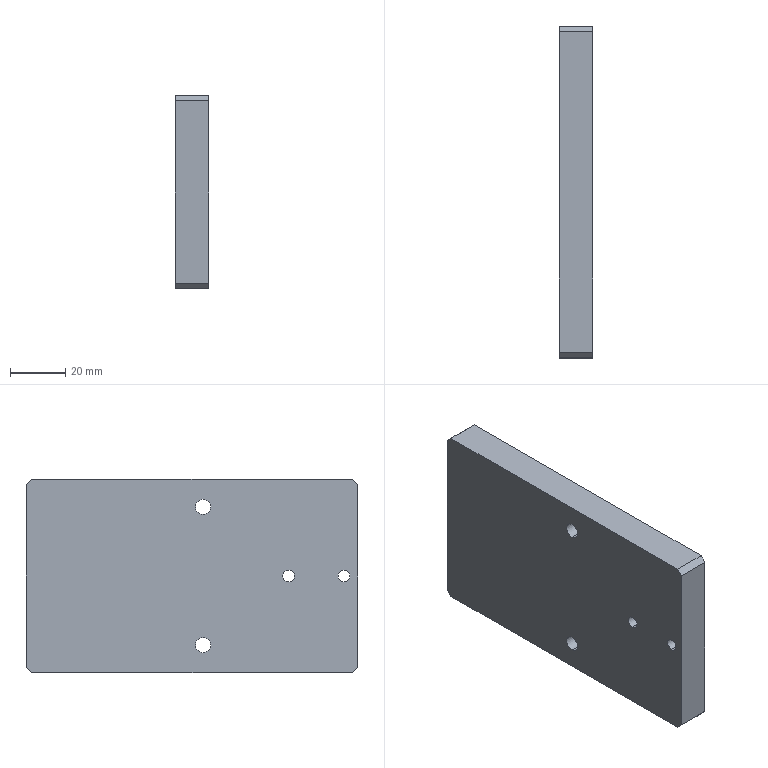Part | SolidWorks | features HoleWzd 4, Chamfer 1, Extrusion 1 | 1 solid | 44 faces | box 12 x 120 x 70 mm | volume 98575 mm3 | cylinder 22 | plane 12 | cone 10 | commonest cylinder face diameters 3.3 x6 4.2 x4 5 x4 5.5 x4 10 x4
STEP:
#1=CARTESIAN_POINT('',(4.,35.5,-26.5));
#2=VERTEX_POINT('',#1);
#3=CARTESIAN_POINT('',(4.,35.5,-31.5));
#4=VERTEX_POINT('',#3);
#5=CARTESIAN_POINT('',(4.,35.5,-29.));
#6=DIRECTION('',(1.,0.,0.));
#7=DIRECTION('',(0.,0.,-1.));
#8=AXIS2_PLACEMENT_3D('',#5,#6,#7);
#9=CIRCLE('',#8,2.5);
#10=EDGE_CURVE('',#2,#4,#9,.T.);
#11=ORIENTED_EDGE('',*,*,#10,.F.);
#12=CARTESIAN_POINT('',(12.,35.5,-26.5));
#13=VERTEX_POINT('',#12);
#14=CARTESIAN_POINT('',(12.,35.5,-26.5));
#15=DIRECTION('',(1.,0.,0.));
#16=VECTOR('',#15,1000.);
#17=LINE('',#14,#16);
#18=EDGE_CURVE('',#2,#13,#17,.T.);
#19=ORIENTED_EDGE('',*,*,#18,.T.);
#20=CARTESIAN_POINT('',(12.,35.5,-31.5));
#21=VERTEX_POINT('',#20);
#22=CARTESIAN_POINT('',(12.,35.5,-29.));
#23=DIRECTION('',(1.,0.,0.));
#24=DIRECTION('',(0.,0.,-1.));
#25=AXIS2_PLACEMENT_3D('',#22,#23,#24);
#26=CIRCLE('',#25,2.5);
#27=EDGE_CURVE('',#13,#21,#26,.T.);
#28=ORIENTED_EDGE('',*,*,#27,.T.);
#29=CARTESIAN_POINT('',(12.,35.5,-31.5));
#30=DIRECTION('',(1.,0.,0.));
#31=VECTOR('',#30,1000.);
#32=LINE('',#29,#31);
#33=EDGE_CURVE('',#4,#21,#32,.T.);
#34=ORIENTED_EDGE('',*,*,#33,.F.);
#35=EDGE_LOOP('',(#11,#19,#28,#34));
#36=FACE_OUTER_BOUND('',#35,.T.);
#37=CARTESIAN_POINT('',(12.,35.5,-29.));
#38=DIRECTION('',(1.,0.,0.));
#39=DIRECTION('',(0.,0.,-1.));
#40=AXIS2_PLACEMENT_3D('',#37,#38,#39);
#41=CYLINDRICAL_SURFACE('',#40,2.5);
#42=ADVANCED_FACE('',(#36),#41,.F.);
#43=CARTESIAN_POINT('',(2.498,35.5,-29.));
#44=VERTEX_POINT('',#43);
#45=CARTESIAN_POINT('',(4.,35.5,-31.5));
#46=DIRECTION('',(0.515,0.,-0.8572));
#47=VECTOR('',#46,1000.);
#48=LINE('',#45,#47);
#49=EDGE_CURVE('',#44,#4,#48,.T.);
#50=ORIENTED_EDGE('',*,*,#49,.F.);
#51=CARTESIAN_POINT('',(4.,35.5,-26.5));
#52=DIRECTION('',(0.515,0.,0.8572));
#53=VECTOR('',#52,1000.);
#54=LINE('',#51,#53);
#55=EDGE_CURVE('',#44,#2,#54,.T.);
#56=ORIENTED_EDGE('',*,*,#55,.T.);
#57=ORIENTED_EDGE('',*,*,#10,.T.);
#58=EDGE_LOOP('',(#50,#56,#57));
#59=FACE_OUTER_BOUND('',#58,.T.);
#60=CARTESIAN_POINT('',(4.,35.5,-29.));
#61=DIRECTION('',(1.,0.,0.));
#62=DIRECTION('',(0.,0.,-1.));
#63=AXIS2_PLACEMENT_3D('',#60,#61,#62);
#64=CONICAL_SURFACE('',#63,2.5,1.03);
#65=ADVANCED_FACE('',(#59),#64,.F.);
#66=CARTESIAN_POINT('',(4.,-12.5,-26.5));
#67=VERTEX_POINT('',#66);
#68=CARTESIAN_POINT('',(4.,-12.5,-31.5));
#69=VERTEX_POINT('',#68);
#70=CARTESIAN_POINT('',(4.,-12.5,-29.));
#71=DIRECTION('',(1.,0.,0.));
#72=DIRECTION('',(0.,0.,-1.));
#73=AXIS2_PLACEMENT_3D('',#70,#71,#72);
#74=CIRCLE('',#73,2.5);
#75=EDGE_CURVE('',#67,#69,#74,.T.);
#76=ORIENTED_EDGE('',*,*,#75,.F.);
#77=CARTESIAN_POINT('',(12.,-12.5,-26.5));
#78=VERTEX_POINT('',#77);
#79=CARTESIAN_POINT('',(12.,-12.5,-26.5));
#80=DIRECTION('',(1.,0.,0.));
#81=VECTOR('',#80,1000.);
#82=LINE('',#79,#81);
#83=EDGE_CURVE('',#67,#78,#82,.T.);
#84=ORIENTED_EDGE('',*,*,#83,.T.);
#85=CARTESIAN_POINT('',(12.,-12.5,-31.5));
#86=VERTEX_POINT('',#85);
#87=CARTESIAN_POINT('',(12.,-12.5,-29.));
#88=DIRECTION('',(1.,0.,0.));
#89=DIRECTION('',(0.,0.,-1.));
#90=AXIS2_PLACEMENT_3D('',#87,#88,#89);
#91=CIRCLE('',#90,2.5);
#92=EDGE_CURVE('',#78,#86,#91,.T.);
#93=ORIENTED_EDGE('',*,*,#92,.T.);
#94=CARTESIAN_POINT('',(12.,-12.5,-31.5));
#95=DIRECTION('',(1.,0.,0.));
#96=VECTOR('',#95,1000.);
#97=LINE('',#94,#96);
#98=EDGE_CURVE('',#69,#86,#97,.T.);
#99=ORIENTED_EDGE('',*,*,#98,.F.);
#100=EDGE_LOOP('',(#76,#84,#93,#99));
#101=FACE_OUTER_BOUND('',#100,.T.);
#102=CARTESIAN_POINT('',(12.,-12.5,-29.));
#103=DIRECTION('',(1.,0.,0.));
#104=DIRECTION('',(0.,0.,-1.));
#105=AXIS2_PLACEMENT_3D('',#102,#103,#104);
#106=CYLINDRICAL_SURFACE('',#105,2.5);
#107=ADVANCED_FACE('',(#101),#106,.F.);
#108=CARTESIAN_POINT('',(2.498,-12.5,-29.));
#109=VERTEX_POINT('',#108);
#110=CARTESIAN_POINT('',(4.,-12.5,-31.5));
#111=DIRECTION('',(0.515,0.,-0.8572));
#112=VECTOR('',#111,1000.);
#113=LINE('',#110,#112);
#114=EDGE_CURVE('',#109,#69,#113,.T.);
#115=ORIENTED_EDGE('',*,*,#114,.F.);
#116=CARTESIAN_POINT('',(4.,-12.5,-26.5));
#117=DIRECTION('',(0.515,0.,0.8572));
#118=VECTOR('',#117,1000.);
#119=LINE('',#116,#118);
#120=EDGE_CURVE('',#109,#67,#119,.T.);
#121=ORIENTED_EDGE('',*,*,#120,.T.);
#122=ORIENTED_EDGE('',*,*,#75,.T.);
#123=EDGE_LOOP('',(#115,#121,#122));
#124=FACE_OUTER_BOUND('',#123,.T.);
#125=CARTESIAN_POINT('',(4.,-12.5,-29.));
#126=DIRECTION('',(1.,0.,0.));
#127=DIRECTION('',(0.,0.,-1.));
#128=AXIS2_PLACEMENT_3D('',#125,#126,#127);
#129=CONICAL_SURFACE('',#128,2.5,1.03);
#130=ADVANCED_FACE('',(#124),#129,.F.);
#131=CARTESIAN_POINT('',(1.9,-48.5,1.65));
#132=VERTEX_POINT('',#131);
#133=CARTESIAN_POINT('',(1.9,-48.5,-1.65));
#134=VERTEX_POINT('',#133);
#135=CARTESIAN_POINT('',(1.9,-48.5,0.));
#136=DIRECTION('',(1.,0.,0.));
#137=DIRECTION('',(0.,0.,-1.));
#138=AXIS2_PLACEMENT_3D('',#135,#136,#137);
#139=CIRCLE('',#138,1.65);
#140=EDGE_CURVE('',#132,#134,#139,.T.);
#141=ORIENTED_EDGE('',*,*,#140,.F.);
#142=CARTESIAN_POINT('',(12.,-48.5,1.65));
#143=VERTEX_POINT('',#142);
#144=CARTESIAN_POINT('',(12.,-48.5,1.65));
#145=DIRECTION('',(1.,0.,0.));
#146=VECTOR('',#145,1000.);
#147=LINE('',#144,#146);
#148=EDGE_CURVE('',#132,#143,#147,.T.);
#149=ORIENTED_EDGE('',*,*,#148,.T.);
#150=CARTESIAN_POINT('',(12.,-48.5,-1.65));
#151=VERTEX_POINT('',#150);
#152=CARTESIAN_POINT('',(12.,-48.5,0.));
#153=DIRECTION('',(1.,0.,0.));
#154=DIRECTION('',(0.,0.,-1.));
#155=AXIS2_PLACEMENT_3D('',#152,#153,#154);
#156=CIRCLE('',#155,1.65);
#157=EDGE_CURVE('',#143,#151,#156,.T.);
#158=ORIENTED_EDGE('',*,*,#157,.T.);
#159=CARTESIAN_POINT('',(12.,-48.5,-1.65));
#160=DIRECTION('',(1.,0.,0.));
#161=VECTOR('',#160,1000.);
#162=LINE('',#159,#161);
#163=EDGE_CURVE('',#134,#151,#162,.T.);
#164=ORIENTED_EDGE('',*,*,#163,.F.);
#165=EDGE_LOOP('',(#141,#149,#158,#164));
#166=FACE_OUTER_BOUND('',#165,.T.);
#167=CARTESIAN_POINT('',(12.,-48.5,0.));
#168=DIRECTION('',(1.,0.,0.));
#169=DIRECTION('',(0.,0.,-1.));
#170=AXIS2_PLACEMENT_3D('',#167,#168,#169);
#171=CYLINDRICAL_SURFACE('',#170,1.65);
#172=ADVANCED_FACE('',(#166),#171,.F.);
#173=CARTESIAN_POINT('',(0.9086,-48.5,0.));
#174=VERTEX_POINT('',#173);
#175=CARTESIAN_POINT('',(1.9,-48.5,-1.65));
#176=DIRECTION('',(0.515,0.,-0.8572));
#177=VECTOR('',#176,1000.);
#178=LINE('',#175,#177);
#179=EDGE_CURVE('',#174,#134,#178,.T.);
#180=ORIENTED_EDGE('',*,*,#179,.F.);
#181=CARTESIAN_POINT('',(1.9,-48.5,1.65));
#182=DIRECTION('',(0.515,0.,0.8572));
#183=VECTOR('',#182,1000.);
#184=LINE('',#181,#183);
#185=EDGE_CURVE('',#174,#132,#184,.T.);
#186=ORIENTED_EDGE('',*,*,#185,.T.);
#187=ORIENTED_EDGE('',*,*,#140,.T.);
#188=EDGE_LOOP('',(#180,#186,#187));
#189=FACE_OUTER_BOUND('',#188,.T.);
#190=CARTESIAN_POINT('',(1.9,-48.5,0.));
#191=DIRECTION('',(1.,0.,0.));
#192=DIRECTION('',(0.,0.,-1.));
#193=AXIS2_PLACEMENT_3D('',#190,#191,#192);
#194=CONICAL_SURFACE('',#193,1.65,1.03);
#195=ADVANCED_FACE('',(#189),#194,.F.);
#196=CARTESIAN_POINT('',(1.9,-12.5,1.65));
#197=VERTEX_POINT('',#196);
#198=CARTESIAN_POINT('',(1.9,-12.5,-1.65));
#199=VERTEX_POINT('',#198);
#200=CARTESIAN_POINT('',(1.9,-12.5,0.));
#201=DIRECTION('',(1.,0.,0.));
#202=DIRECTION('',(0.,0.,-1.));
#203=AXIS2_PLACEMENT_3D('',#200,#201,#202);
#204=CIRCLE('',#203,1.65);
#205=EDGE_CURVE('',#197,#199,#204,.T.);
#206=ORIENTED_EDGE('',*,*,#205,.F.);
#207=CARTESIAN_POINT('',(12.,-12.5,1.65));
#208=VERTEX_POINT('',#207);
#209=CARTESIAN_POINT('',(12.,-12.5,1.65));
#210=DIRECTION('',(1.,0.,0.));
#211=VECTOR('',#210,1000.);
#212=LINE('',#209,#211);
#213=EDGE_CURVE('',#197,#208,#212,.T.);
#214=ORIENTED_EDGE('',*,*,#213,.T.);
#215=CARTESIAN_POINT('',(12.,-12.5,-1.65));
#216=VERTEX_POINT('',#215);
#217=CARTESIAN_POINT('',(12.,-12.5,0.));
#218=DIRECTION('',(1.,0.,0.));
#219=DIRECTION('',(0.,0.,-1.));
#220=AXIS2_PLACEMENT_3D('',#217,#218,#219);
#221=CIRCLE('',#220,1.65);
#222=EDGE_CURVE('',#208,#216,#221,.T.);
#223=ORIENTED_EDGE('',*,*,#222,.T.);
#224=CARTESIAN_POINT('',(12.,-12.5,-1.65));
#225=DIRECTION('',(1.,0.,0.));
#226=VECTOR('',#225,1000.);
#227=LINE('',#224,#226);
#228=EDGE_CURVE('',#199,#216,#227,.T.);
#229=ORIENTED_EDGE('',*,*,#228,.F.);
#230=EDGE_LOOP('',(#206,#214,#223,#229));
#231=FACE_OUTER_BOUND('',#230,.T.);
#232=CARTESIAN_POINT('',(12.,-12.5,0.));
#233=DIRECTION('',(1.,0.,0.));
#234=DIRECTION('',(0.,0.,-1.));
#235=AXIS2_PLACEMENT_3D('',#232,#233,#234);
#236=CYLINDRICAL_SURFACE('',#235,1.65);
#237=ADVANCED_FACE('',(#231),#236,.F.);
#238=CARTESIAN_POINT('',(0.9086,-12.5,0.));
#239=VERTEX_POINT('',#238);
#240=CARTESIAN_POINT('',(1.9,-12.5,-1.65));
#241=DIRECTION('',(0.515,0.,-0.8572));
#242=VECTOR('',#241,1000.);
#243=LINE('',#240,#242);
#244=EDGE_CURVE('',#239,#199,#243,.T.);
#245=ORIENTED_EDGE('',*,*,#244,.F.);
#246=CARTESIAN_POINT('',(1.9,-12.5,1.65));
#247=DIRECTION('',(0.515,0.,0.8572));
#248=VECTOR('',#247,1000.);
#249=LINE('',#246,#248);
#250=EDGE_CURVE('',#239,#197,#249,.T.);
#251=ORIENTED_EDGE('',*,*,#250,.T.);
#252=ORIENTED_EDGE('',*,*,#205,.T.);
#253=EDGE_LOOP('',(#245,#251,#252));
#254=FACE_OUTER_BOUND('',#253,.T.);
#255=CARTESIAN_POINT('',(1.9,-12.5,0.));
#256=DIRECTION('',(1.,0.,0.));
#257=DIRECTION('',(0.,0.,-1.));
#258=AXIS2_PLACEMENT_3D('',#255,#256,#257);
#259=CONICAL_SURFACE('',#258,1.65,1.03);
#260=ADVANCED_FACE('',(#254),#259,.F.);
#261=CARTESIAN_POINT('',(1.9,35.5,1.65));
#262=VERTEX_POINT('',#261);
#263=CARTESIAN_POINT('',(1.9,35.5,-1.65));
#264=VERTEX_POINT('',#263);
#265=CARTESIAN_POINT('',(1.9,35.5,0.));
#266=DIRECTION('',(1.,0.,0.));
#267=DIRECTION('',(0.,0.,-1.));
#268=AXIS2_PLACEMENT_3D('',#265,#266,#267);
#269=CIRCLE('',#268,1.65);
#270=EDGE_CURVE('',#262,#264,#269,.T.);
#271=ORIENTED_EDGE('',*,*,#270,.F.);
#272=CARTESIAN_POINT('',(12.,35.5,1.65));
#273=VERTEX_POINT('',#272);
#274=CARTESIAN_POINT('',(12.,35.5,1.65));
#275=DIRECTION('',(1.,0.,0.));
#276=VECTOR('',#275,1000.);
#277=LINE('',#274,#276);
#278=EDGE_CURVE('',#262,#273,#277,.T.);
#279=ORIENTED_EDGE('',*,*,#278,.T.);
#280=CARTESIAN_POINT('',(12.,35.5,-1.65));
#281=VERTEX_POINT('',#280);
#282=CARTESIAN_POINT('',(12.,35.5,0.));
#283=DIRECTION('',(1.,0.,0.));
#284=DIRECTION('',(0.,0.,-1.));
#285=AXIS2_PLACEMENT_3D('',#282,#283,#284);
#286=CIRCLE('',#285,1.65);
#287=EDGE_CURVE('',#273,#281,#286,.T.);
#288=ORIENTED_EDGE('',*,*,#287,.T.);
#289=CARTESIAN_POINT('',(12.,35.5,-1.65));
#290=DIRECTION('',(1.,0.,0.));
#291=VECTOR('',#290,1000.);
#292=LINE('',#289,#291);
#293=EDGE_CURVE('',#264,#281,#292,.T.);
#294=ORIENTED_EDGE('',*,*,#293,.F.);
#295=EDGE_LOOP('',(#271,#279,#288,#294));
#296=FACE_OUTER_BOUND('',#295,.T.);
#297=CARTESIAN_POINT('',(12.,35.5,0.));
#298=DIRECTION('',(1.,0.,0.));
#299=DIRECTION('',(0.,0.,-1.));
#300=AXIS2_PLACEMENT_3D('',#297,#298,#299);
#301=CYLINDRICAL_SURFACE('',#300,1.65);
#302=ADVANCED_FACE('',(#296),#301,.F.);
#303=CARTESIAN_POINT('',(0.9086,35.5,0.));
#304=VERTEX_POINT('',#303);
#305=CARTESIAN_POINT('',(1.9,35.5,-1.65));
#306=DIRECTION('',(0.515,0.,-0.8572));
#307=VECTOR('',#306,1000.);
#308=LINE('',#305,#307);
#309=EDGE_CURVE('',#304,#264,#308,.T.);
#310=ORIENTED_EDGE('',*,*,#309,.F.);
#311=CARTESIAN_POINT('',(1.9,35.5,1.65));
#312=DIRECTION('',(0.515,0.,0.8572));
#313=VECTOR('',#312,1000.);
#314=LINE('',#311,#313);
#315=EDGE_CURVE('',#304,#262,#314,.T.);
#316=ORIENTED_EDGE('',*,*,#315,.T.);
#317=ORIENTED_EDGE('',*,*,#270,.T.);
#318=EDGE_LOOP('',(#310,#316,#317));
#319=FACE_OUTER_BOUND('',#318,.T.);
#320=CARTESIAN_POINT('',(1.9,35.5,0.));
#321=DIRECTION('',(1.,0.,0.));
#322=DIRECTION('',(0.,0.,-1.));
#323=AXIS2_PLACEMENT_3D('',#320,#321,#322);
#324=CONICAL_SURFACE('',#323,1.65,1.03);
#325=ADVANCED_FACE('',(#319),#324,.F.);
#326=CARTESIAN_POINT('',(6.3,-4.,-20.));
#327=VERTEX_POINT('',#326);
#328=CARTESIAN_POINT('',(6.3,-4.,-30.));
#329=VERTEX_POINT('',#328);
#330=CARTESIAN_POINT('',(6.3,-4.,-25.));
#331=DIRECTION('',(1.,0.,0.));
#332=DIRECTION('',(0.,0.,-1.));
#333=AXIS2_PLACEMENT_3D('',#330,#331,#332);
#334=CIRCLE('',#333,5.);
#335=EDGE_CURVE('',#327,#329,#334,.T.);
#336=ORIENTED_EDGE('',*,*,#335,.F.);
#337=CARTESIAN_POINT('',(12.,-4.,-20.));
#338=VERTEX_POINT('',#337);
#339=CARTESIAN_POINT('',(12.,-4.,-20.));
#340=DIRECTION('',(1.,0.,0.));
#341=VECTOR('',#340,1000.);
#342=LINE('',#339,#341);
#343=EDGE_CURVE('',#327,#338,#342,.T.);
#344=ORIENTED_EDGE('',*,*,#343,.T.);
#345=CARTESIAN_POINT('',(12.,-4.,-30.));
#346=VERTEX_POINT('',#345);
#347=CARTESIAN_POINT('',(12.,-4.,-25.));
#348=DIRECTION('',(1.,0.,0.));
#349=DIRECTION('',(0.,0.,-1.));
#350=AXIS2_PLACEMENT_3D('',#347,#348,#349);
#351=CIRCLE('',#350,5.);
#352=EDGE_CURVE('',#338,#346,#351,.T.);
#353=ORIENTED_EDGE('',*,*,#352,.T.);
#354=CARTESIAN_POINT('',(12.,-4.,-30.));
#355=DIRECTION('',(1.,0.,0.));
#356=VECTOR('',#355,1000.);
#357=LINE('',#354,#356);
#358=EDGE_CURVE('',#329,#346,#357,.T.);
#359=ORIENTED_EDGE('',*,*,#358,.F.);
#360=EDGE_LOOP('',(#336,#344,#353,#359));
#361=FACE_OUTER_BOUND('',#360,.T.);
#362=CARTESIAN_POINT('',(12.,-4.,-25.));
#363=DIRECTION('',(1.,0.,0.));
#364=DIRECTION('',(0.,0.,-1.));
#365=AXIS2_PLACEMENT_3D('',#362,#363,#364);
#366=CYLINDRICAL_SURFACE('',#365,5.);
#367=ADVANCED_FACE('',(#361),#366,.F.);
#368=CARTESIAN_POINT('',(0.,-4.,-22.25));
#369=VERTEX_POINT('',#368);
#370=CARTESIAN_POINT('',(0.,-4.,-27.75));
#371=VERTEX_POINT('',#370);
#372=CARTESIAN_POINT('',(0.,-4.,-25.));
#373=DIRECTION('',(1.,0.,0.));
#374=DIRECTION('',(0.,0.,-1.));
#375=AXIS2_PLACEMENT_3D('',#372,#373,#374);
#376=CIRCLE('',#375,2.75);
#377=EDGE_CURVE('',#369,#371,#376,.T.);
#378=ORIENTED_EDGE('',*,*,#377,.F.);
#379=CARTESIAN_POINT('',(6.3,-4.,-22.25));
#380=VERTEX_POINT('',#379);
#381=CARTESIAN_POINT('',(12.,-4.,-22.25));
#382=DIRECTION('',(1.,0.,0.));
#383=VECTOR('',#382,1000.);
#384=LINE('',#381,#383);
#385=EDGE_CURVE('',#369,#380,#384,.T.);
#386=ORIENTED_EDGE('',*,*,#385,.T.);
#387=CARTESIAN_POINT('',(6.3,-4.,-27.75));
#388=VERTEX_POINT('',#387);
#389=CARTESIAN_POINT('',(6.3,-4.,-25.));
#390=DIRECTION('',(1.,0.,0.));
#391=DIRECTION('',(0.,0.,-1.));
#392=AXIS2_PLACEMENT_3D('',#389,#390,#391);
#393=CIRCLE('',#392,2.75);
#394=EDGE_CURVE('',#380,#388,#393,.T.);
#395=ORIENTED_EDGE('',*,*,#394,.T.);
#396=CARTESIAN_POINT('',(12.,-4.,-27.75));
#397=DIRECTION('',(1.,0.,0.));
#398=VECTOR('',#397,1000.);
#399=LINE('',#396,#398);
#400=EDGE_CURVE('',#371,#388,#399,.T.);
#401=ORIENTED_EDGE('',*,*,#400,.F.);
#402=EDGE_LOOP('',(#378,#386,#395,#401));
#403=FACE_OUTER_BOUND('',#402,.T.);
#404=CARTESIAN_POINT('',(12.,-4.,-25.));
#405=DIRECTION('',(1.,0.,0.));
#406=DIRECTION('',(0.,0.,-1.));
#407=AXIS2_PLACEMENT_3D('',#404,#405,#406);
#408=CYLINDRICAL_SURFACE('',#407,2.75);
#409=ADVANCED_FACE('',(#403),#408,.F.);
#410=CARTESIAN_POINT('',(6.3,-4.,30.));
#411=VERTEX_POINT('',#410);
#412=CARTESIAN_POINT('',(6.3,-4.,20.));
#413=VERTEX_POINT('',#412);
#414=CARTESIAN_POINT('',(6.3,-4.,25.));
#415=DIRECTION('',(1.,0.,0.));
#416=DIRECTION('',(0.,0.,-1.));
#417=AXIS2_PLACEMENT_3D('',#414,#415,#416);
#418=CIRCLE('',#417,5.);
#419=EDGE_CURVE('',#411,#413,#418,.T.);
#420=ORIENTED_EDGE('',*,*,#419,.F.);
#421=CARTESIAN_POINT('',(12.,-4.,30.));
#422=VERTEX_POINT('',#421);
#423=CARTESIAN_POINT('',(12.,-4.,30.));
#424=DIRECTION('',(1.,0.,0.));
#425=VECTOR('',#424,1000.);
#426=LINE('',#423,#425);
#427=EDGE_CURVE('',#411,#422,#426,.T.);
#428=ORIENTED_EDGE('',*,*,#427,.T.);
#429=CARTESIAN_POINT('',(12.,-4.,20.));
#430=VERTEX_POINT('',#429);
#431=CARTESIAN_POINT('',(12.,-4.,25.));
#432=DIRECTION('',(1.,0.,0.));
#433=DIRECTION('',(0.,0.,-1.));
#434=AXIS2_PLACEMENT_3D('',#431,#432,#433);
#435=CIRCLE('',#434,5.);
#436=EDGE_CURVE('',#422,#430,#435,.T.);
#437=ORIENTED_EDGE('',*,*,#436,.T.);
#438=CARTESIAN_POINT('',(12.,-4.,20.));
#439=DIRECTION('',(1.,0.,0.));
#440=VECTOR('',#439,1000.);
#441=LINE('',#438,#440);
#442=EDGE_CURVE('',#413,#430,#441,.T.);
#443=ORIENTED_EDGE('',*,*,#442,.F.);
#444=EDGE_LOOP('',(#420,#428,#437,#443));
#445=FACE_OUTER_BOUND('',#444,.T.);
#446=CARTESIAN_POINT('',(12.,-4.,25.));
#447=DIRECTION('',(1.,0.,0.));
#448=DIRECTION('',(0.,0.,-1.));
#449=AXIS2_PLACEMENT_3D('',#446,#447,#448);
#450=CYLINDRICAL_SURFACE('',#449,5.);
#451=ADVANCED_FACE('',(#445),#450,.F.);
#452=CARTESIAN_POINT('',(0.,-4.,27.75));
#453=VERTEX_POINT('',#452);
#454=CARTESIAN_POINT('',(0.,-4.,22.25));
#455=VERTEX_POINT('',#454);
#456=CARTESIAN_POINT('',(0.,-4.,25.));
#457=DIRECTION('',(1.,0.,0.));
#458=DIRECTION('',(0.,0.,-1.));
#459=AXIS2_PLACEMENT_3D('',#456,#457,#458);
#460=CIRCLE('',#459,2.75);
#461=EDGE_CURVE('',#453,#455,#460,.T.);
#462=ORIENTED_EDGE('',*,*,#461,.F.);
#463=CARTESIAN_POINT('',(6.3,-4.,27.75));
#464=VERTEX_POINT('',#463);
#465=CARTESIAN_POINT('',(12.,-4.,27.75));
#466=DIRECTION('',(1.,0.,0.));
#467=VECTOR('',#466,1000.);
#468=LINE('',#465,#467);
#469=EDGE_CURVE('',#453,#464,#468,.T.);
#470=ORIENTED_EDGE('',*,*,#469,.T.);
#471=CARTESIAN_POINT('',(6.3,-4.,22.25));
#472=VERTEX_POINT('',#471);
#473=CARTESIAN_POINT('',(6.3,-4.,25.));
#474=DIRECTION('',(1.,0.,0.));
#475=DIRECTION('',(0.,0.,-1.));
#476=AXIS2_PLACEMENT_3D('',#473,#474,#475);
#477=CIRCLE('',#476,2.75);
#478=EDGE_CURVE('',#464,#472,#477,.T.);
#479=ORIENTED_EDGE('',*,*,#478,.T.);
#480=CARTESIAN_POINT('',(12.,-4.,22.25));
#481=DIRECTION('',(1.,0.,0.));
#482=VECTOR('',#481,1000.);
#483=LINE('',#480,#482);
#484=EDGE_CURVE('',#455,#472,#483,.T.);
#485=ORIENTED_EDGE('',*,*,#484,.F.);
#486=EDGE_LOOP('',(#462,#470,#479,#485));
#487=FACE_OUTER_BOUND('',#486,.T.);
#488=CARTESIAN_POINT('',(12.,-4.,25.));
#489=DIRECTION('',(1.,0.,0.));
#490=DIRECTION('',(0.,0.,-1.));
#491=AXIS2_PLACEMENT_3D('',#488,#489,#490);
#492=CYLINDRICAL_SURFACE('',#491,2.75);
#493=ADVANCED_FACE('',(#487),#492,.F.);
#494=CARTESIAN_POINT('',(12.,-35.,-2.1));
#495=VERTEX_POINT('',#494);
#496=CARTESIAN_POINT('',(12.,-35.,2.1));
#497=VERTEX_POINT('',#496);
#498=CARTESIAN_POINT('',(12.,-35.,0.));
#499=DIRECTION('',(-1.,0.,0.));
#500=DIRECTION('',(0.,0.,1.));
#501=AXIS2_PLACEMENT_3D('',#498,#499,#500);
#502=CIRCLE('',#501,2.1);
#503=EDGE_CURVE('',#495,#497,#502,.T.);
#504=ORIENTED_EDGE('',*,*,#503,.F.);
#505=CARTESIAN_POINT('',(0.,-35.,-2.1));
#506=VERTEX_POINT('',#505);
#507=CARTESIAN_POINT('',(0.,-35.,-2.1));
#508=DIRECTION('',(-1.,0.,0.));
#509=VECTOR('',#508,1000.);
#510=LINE('',#507,#509);
#511=EDGE_CURVE('',#495,#506,#510,.T.);
#512=ORIENTED_EDGE('',*,*,#511,.T.);
#513=CARTESIAN_POINT('',(0.,-35.,2.1));
#514=VERTEX_POINT('',#513);
#515=CARTESIAN_POINT('',(0.,-35.,0.));
#516=DIRECTION('',(-1.,0.,0.));
#517=DIRECTION('',(0.,0.,1.));
#518=AXIS2_PLACEMENT_3D('',#515,#516,#517);
#519=CIRCLE('',#518,2.1);
#520=EDGE_CURVE('',#506,#514,#519,.T.);
#521=ORIENTED_EDGE('',*,*,#520,.T.);
#522=CARTESIAN_POINT('',(0.,-35.,2.1));
#523=DIRECTION('',(-1.,0.,0.));
#524=VECTOR('',#523,1000.);
#525=LINE('',#522,#524);
#526=EDGE_CURVE('',#497,#514,#525,.T.);
#527=ORIENTED_EDGE('',*,*,#526,.F.);
#528=EDGE_LOOP('',(#504,#512,#521,#527));
#529=FACE_OUTER_BOUND('',#528,.T.);
#530=CARTESIAN_POINT('',(0.,-35.,0.));
#531=DIRECTION('',(-1.,0.,0.));
#532=DIRECTION('',(0.,0.,1.));
#533=AXIS2_PLACEMENT_3D('',#530,#531,#532);
#534=CYLINDRICAL_SURFACE('',#533,2.1);
#535=ADVANCED_FACE('',(#529),#534,.F.);
#536=CARTESIAN_POINT('',(12.,-55.,-2.1));
#537=VERTEX_POINT('',#536);
#538=CARTESIAN_POINT('',(12.,-55.,2.1));
#539=VERTEX_POINT('',#538);
#540=CARTESIAN_POINT('',(12.,-55.,0.));
#541=DIRECTION('',(-1.,0.,0.));
#542=DIRECTION('',(0.,0.,1.));
#543=AXIS2_PLACEMENT_3D('',#540,#541,#542);
#544=CIRCLE('',#543,2.1);
#545=EDGE_CURVE('',#537,#539,#544,.T.);
#546=ORIENTED_EDGE('',*,*,#545,.F.);
#547=CARTESIAN_POINT('',(0.,-55.,-2.1));
#548=VERTEX_POINT('',#547);
#549=CARTESIAN_POINT('',(0.,-55.,-2.1));
#550=DIRECTION('',(-1.,0.,0.));
#551=VECTOR('',#550,1000.);
#552=LINE('',#549,#551);
#553=EDGE_CURVE('',#537,#548,#552,.T.);
#554=ORIENTED_EDGE('',*,*,#553,.T.);
#555=CARTESIAN_POINT('',(0.,-55.,2.1));
#556=VERTEX_POINT('',#555);
#557=CARTESIAN_POINT('',(0.,-55.,0.));
#558=DIRECTION('',(-1.,0.,0.));
#559=DIRECTION('',(0.,0.,1.));
#560=AXIS2_PLACEMENT_3D('',#557,#558,#559);
#561=CIRCLE('',#560,2.1);
#562=EDGE_CURVE('',#548,#556,#561,.T.);
#563=ORIENTED_EDGE('',*,*,#562,.T.);
#564=CARTESIAN_POINT('',(0.,-55.,2.1));
#565=DIRECTION('',(-1.,0.,0.));
#566=VECTOR('',#565,1000.);
#567=LINE('',#564,#566);
#568=EDGE_CURVE('',#539,#556,#567,.T.);
#569=ORIENTED_EDGE('',*,*,#568,.F.);
#570=EDGE_LOOP('',(#546,#554,#563,#569));
#571=FACE_OUTER_BOUND('',#570,.T.);
#572=CARTESIAN_POINT('',(0.,-55.,0.));
#573=DIRECTION('',(-1.,0.,0.));
#574=DIRECTION('',(0.,0.,1.));
#575=AXIS2_PLACEMENT_3D('',#572,#573,#574);
#576=CYLINDRICAL_SURFACE('',#575,2.1);
#577=ADVANCED_FACE('',(#571),#576,.F.);
#578=CARTESIAN_POINT('',(12.,-58.,-35.));
#579=VERTEX_POINT('',#578);
#580=CARTESIAN_POINT('',(12.,58.,-35.));
#581=VERTEX_POINT('',#580);
#582=CARTESIAN_POINT('',(12.,-60.,-35.));
#583=DIRECTION('',(0.,1.,0.));
#584=VECTOR('',#583,1000.);
#585=LINE('',#582,#584);
#586=EDGE_CURVE('',#579,#581,#585,.T.);
#587=ORIENTED_EDGE('',*,*,#586,.F.);
#588=CARTESIAN_POINT('',(0.,-58.,-35.));
#589=VERTEX_POINT('',#588);
#590=CARTESIAN_POINT('',(12.,-58.,-35.));
#591=DIRECTION('',(-1.,0.,0.));
#592=VECTOR('',#591,1000.);
#593=LINE('',#590,#592);
#594=EDGE_CURVE('',#579,#589,#593,.T.);
#595=ORIENTED_EDGE('',*,*,#594,.T.);
#596=CARTESIAN_POINT('',(0.,58.,-35.));
#597=VERTEX_POINT('',#596);
#598=CARTESIAN_POINT('',(0.,-60.,-35.));
#599=DIRECTION('',(0.,1.,0.));
#600=VECTOR('',#599,1000.);
#601=LINE('',#598,#600);
#602=EDGE_CURVE('',#589,#597,#601,.T.);
#603=ORIENTED_EDGE('',*,*,#602,.T.);
#604=CARTESIAN_POINT('',(12.,58.,-35.));
#605=DIRECTION('',(1.,0.,0.));
#606=VECTOR('',#605,1000.);
#607=LINE('',#604,#606);
#608=EDGE_CURVE('',#597,#581,#607,.T.);
#609=ORIENTED_EDGE('',*,*,#608,.T.);
#610=EDGE_LOOP('',(#587,#595,#603,#609));
#611=FACE_OUTER_BOUND('',#610,.T.);
#612=CARTESIAN_POINT('',(12.,-60.,-35.));
#613=DIRECTION('',(0.,0.,1.));
#614=DIRECTION('',(1.,0.,0.));
#615=AXIS2_PLACEMENT_3D('',#612,#613,#614);
#616=PLANE('',#615);
#617=ADVANCED_FACE('',(#611),#616,.F.);
#618=CARTESIAN_POINT('',(12.,60.,-33.));
#619=VERTEX_POINT('',#618);
#620=CARTESIAN_POINT('',(12.,60.,33.));
#621=VERTEX_POINT('',#620);
#622=CARTESIAN_POINT('',(12.,60.,35.));
#623=DIRECTION('',(0.,0.,1.));
#624=VECTOR('',#623,1000.);
#625=LINE('',#622,#624);
#626=EDGE_CURVE('',#619,#621,#625,.T.);
#627=ORIENTED_EDGE('',*,*,#626,.F.);
#628=CARTESIAN_POINT('',(0.,60.,-33.));
#629=VERTEX_POINT('',#628);
#630=CARTESIAN_POINT('',(12.,60.,-33.));
#631=DIRECTION('',(-1.,0.,0.));
#632=VECTOR('',#631,1000.);
#633=LINE('',#630,#632);
#634=EDGE_CURVE('',#619,#629,#633,.T.);
#635=ORIENTED_EDGE('',*,*,#634,.T.);
#636=CARTESIAN_POINT('',(0.,60.,33.));
#637=VERTEX_POINT('',#636);
#638=CARTESIAN_POINT('',(0.,60.,35.));
#639=DIRECTION('',(0.,0.,1.));
#640=VECTOR('',#639,1000.);
#641=LINE('',#638,#640);
#642=EDGE_CURVE('',#629,#637,#641,.T.);
#643=ORIENTED_EDGE('',*,*,#642,.T.);
#644=CARTESIAN_POINT('',(12.,60.,33.));
#645=DIRECTION('',(1.,0.,0.));
#646=VECTOR('',#645,1000.);
#647=LINE('',#644,#646);
#648=EDGE_CURVE('',#637,#621,#647,.T.);
#649=ORIENTED_EDGE('',*,*,#648,.T.);
#650=EDGE_LOOP('',(#627,#635,#643,#649));
#651=FACE_OUTER_BOUND('',#650,.T.);
#652=CARTESIAN_POINT('',(12.,60.,35.));
#653=DIRECTION('',(0.,-1.,0.));
#654=DIRECTION('',(0.,0.,-1.));
#655=AXIS2_PLACEMENT_3D('',#652,#653,#654);
#656=PLANE('',#655);
#657=ADVANCED_FACE('',(#651),#656,.F.);
#658=CARTESIAN_POINT('',(0.,58.,35.));
#659=VERTEX_POINT('',#658);
#660=CARTESIAN_POINT('',(0.,-58.,35.));
#661=VERTEX_POINT('',#660);
#662=CARTESIAN_POINT('',(0.,-60.,35.));
#663=DIRECTION('',(0.,-1.,0.));
#664=VECTOR('',#663,1000.);
#665=LINE('',#662,#664);
#666=EDGE_CURVE('',#659,#661,#665,.T.);
#667=ORIENTED_EDGE('',*,*,#666,.T.);
#668=CARTESIAN_POINT('',(12.,-58.,35.));
#669=VERTEX_POINT('',#668);
#670=CARTESIAN_POINT('',(12.,-58.,35.));
#671=DIRECTION('',(1.,0.,0.));
#672=VECTOR('',#671,1000.);
#673=LINE('',#670,#672);
#674=EDGE_CURVE('',#661,#669,#673,.T.);
#675=ORIENTED_EDGE('',*,*,#674,.T.);
#676=CARTESIAN_POINT('',(12.,58.,35.));
#677=VERTEX_POINT('',#676);
#678=CARTESIAN_POINT('',(12.,-60.,35.));
#679=DIRECTION('',(0.,-1.,0.));
#680=VECTOR('',#679,1000.);
#681=LINE('',#678,#680);
#682=EDGE_CURVE('',#677,#669,#681,.T.);
#683=ORIENTED_EDGE('',*,*,#682,.F.);
#684=CARTESIAN_POINT('',(12.,58.,35.));
#685=DIRECTION('',(-1.,0.,0.));
#686=VECTOR('',#685,1000.);
#687=LINE('',#684,#686);
#688=EDGE_CURVE('',#677,#659,#687,.T.);
#689=ORIENTED_EDGE('',*,*,#688,.T.);
#690=EDGE_LOOP('',(#667,#675,#683,#689));
#691=FACE_OUTER_BOUND('',#690,.T.);
#692=CARTESIAN_POINT('',(12.,-60.,35.));
#693=DIRECTION('',(0.,0.,-1.));
#694=DIRECTION('',(-1.,0.,0.));
#695=AXIS2_PLACEMENT_3D('',#692,#693,#694);
#696=PLANE('',#695);
#697=ADVANCED_FACE('',(#691),#696,.F.);
#698=CARTESIAN_POINT('',(0.,-60.,33.));
#699=VERTEX_POINT('',#698);
#700=CARTESIAN_POINT('',(0.,-60.,-33.));
#701=VERTEX_POINT('',#700);
#702=CARTESIAN_POINT('',(0.,-60.,35.));
#703=DIRECTION('',(0.,0.,-1.));
#704=VECTOR('',#703,1000.);
#705=LINE('',#702,#704);
#706=EDGE_CURVE('',#699,#701,#705,.T.);
#707=ORIENTED_EDGE('',*,*,#706,.T.);
#708=CARTESIAN_POINT('',(12.,-60.,-33.));
#709=VERTEX_POINT('',#708);
#710=CARTESIAN_POINT('',(12.,-60.,-33.));
#711=DIRECTION('',(1.,0.,0.));
#712=VECTOR('',#711,1000.);
#713=LINE('',#710,#712);
#714=EDGE_CURVE('',#701,#709,#713,.T.);
#715=ORIENTED_EDGE('',*,*,#714,.T.);
#716=CARTESIAN_POINT('',(12.,-60.,33.));
#717=VERTEX_POINT('',#716);
#718=CARTESIAN_POINT('',(12.,-60.,35.));
#719=DIRECTION('',(0.,0.,-1.));
#720=VECTOR('',#719,1000.);
#721=LINE('',#718,#720);
#722=EDGE_CURVE('',#717,#709,#721,.T.);
#723=ORIENTED_EDGE('',*,*,#722,.F.);
#724=CARTESIAN_POINT('',(12.,-60.,33.));
#725=DIRECTION('',(-1.,0.,0.));
#726=VECTOR('',#725,1000.);
#727=LINE('',#724,#726);
#728=EDGE_CURVE('',#717,#699,#727,.T.);
#729=ORIENTED_EDGE('',*,*,#728,.T.);
#730=EDGE_LOOP('',(#707,#715,#723,#729));
#731=FACE_OUTER_BOUND('',#730,.T.);
#732=CARTESIAN_POINT('',(12.,-60.,35.));
#733=DIRECTION('',(0.,1.,0.));
#734=DIRECTION('',(0.,0.,1.));
#735=AXIS2_PLACEMENT_3D('',#732,#733,#734);
#736=PLANE('',#735);
#737=ADVANCED_FACE('',(#731),#736,.F.);
#738=CARTESIAN_POINT('',(12.,35.5,-29.));
#739=DIRECTION('',(1.,0.,0.));
#740=DIRECTION('',(0.,0.,-1.));
#741=AXIS2_PLACEMENT_3D('',#738,#739,#740);
#742=CIRCLE('',#741,2.5);
#743=EDGE_CURVE('',#21,#13,#742,.T.);
#744=ORIENTED_EDGE('',*,*,#743,.F.);
#745=ORIENTED_EDGE('',*,*,#27,.F.);
#746=EDGE_LOOP('',(#744,#745));
#747=FACE_BOUND('',#746,.T.);
#748=CARTESIAN_POINT('',(12.,-12.5,-29.));
#749=DIRECTION('',(1.,0.,0.));
#750=DIRECTION('',(0.,0.,-1.));
#751=AXIS2_PLACEMENT_3D('',#748,#749,#750);
#752=CIRCLE('',#751,2.5);
#753=EDGE_CURVE('',#86,#78,#752,.T.);
#754=ORIENTED_EDGE('',*,*,#753,.F.);
#755=ORIENTED_EDGE('',*,*,#92,.F.);
#756=EDGE_LOOP('',(#754,#755));
#757=FACE_BOUND('',#756,.T.);
#758=CARTESIAN_POINT('',(12.,-48.5,0.));
#759=DIRECTION('',(1.,0.,0.));
#760=DIRECTION('',(0.,0.,-1.));
#761=AXIS2_PLACEMENT_3D('',#758,#759,#760);
#762=CIRCLE('',#761,1.65);
#763=EDGE_CURVE('',#151,#143,#762,.T.);
#764=ORIENTED_EDGE('',*,*,#763,.F.);
#765=ORIENTED_EDGE('',*,*,#157,.F.);
#766=EDGE_LOOP('',(#764,#765));
#767=FACE_BOUND('',#766,.T.);
#768=CARTESIAN_POINT('',(12.,-12.5,0.));
#769=DIRECTION('',(1.,0.,0.));
#770=DIRECTION('',(0.,0.,-1.));
#771=AXIS2_PLACEMENT_3D('',#768,#769,#770);
#772=CIRCLE('',#771,1.65);
#773=EDGE_CURVE('',#216,#208,#772,.T.);
#774=ORIENTED_EDGE('',*,*,#773,.F.);
#775=ORIENTED_EDGE('',*,*,#222,.F.);
#776=EDGE_LOOP('',(#774,#775));
#777=FACE_BOUND('',#776,.T.);
#778=CARTESIAN_POINT('',(12.,35.5,0.));
#779=DIRECTION('',(1.,0.,0.));
#780=DIRECTION('',(0.,0.,-1.));
#781=AXIS2_PLACEMENT_3D('',#778,#779,#780);
#782=CIRCLE('',#781,1.65);
#783=EDGE_CURVE('',#281,#273,#782,.T.);
#784=ORIENTED_EDGE('',*,*,#783,.F.);
#785=ORIENTED_EDGE('',*,*,#287,.F.);
#786=EDGE_LOOP('',(#784,#785));
#787=FACE_BOUND('',#786,.T.);
#788=CARTESIAN_POINT('',(12.,-4.,-25.));
#789=DIRECTION('',(1.,0.,0.));
#790=DIRECTION('',(0.,0.,-1.));
#791=AXIS2_PLACEMENT_3D('',#788,#789,#790);
#792=CIRCLE('',#791,5.);
#793=EDGE_CURVE('',#346,#338,#792,.T.);
#794=ORIENTED_EDGE('',*,*,#793,.F.);
#795=ORIENTED_EDGE('',*,*,#352,.F.);
#796=EDGE_LOOP('',(#794,#795));
#797=FACE_BOUND('',#796,.T.);
#798=CARTESIAN_POINT('',(12.,-4.,25.));
#799=DIRECTION('',(1.,0.,0.));
#800=DIRECTION('',(0.,0.,-1.));
#801=AXIS2_PLACEMENT_3D('',#798,#799,#800);
#802=CIRCLE('',#801,5.);
#803=EDGE_CURVE('',#430,#422,#802,.T.);
#804=ORIENTED_EDGE('',*,*,#803,.F.);
#805=ORIENTED_EDGE('',*,*,#436,.F.);
#806=EDGE_LOOP('',(#804,#805));
#807=FACE_BOUND('',#806,.T.);
#808=CARTESIAN_POINT('',(12.,-35.,0.));
#809=DIRECTION('',(-1.,0.,0.));
#810=DIRECTION('',(0.,0.,1.));
#811=AXIS2_PLACEMENT_3D('',#808,#809,#810);
#812=CIRCLE('',#811,2.1);
#813=EDGE_CURVE('',#497,#495,#812,.T.);
#814=ORIENTED_EDGE('',*,*,#813,.T.);
#815=ORIENTED_EDGE('',*,*,#503,.T.);
#816=EDGE_LOOP('',(#814,#815));
#817=FACE_BOUND('',#816,.T.);
#818=CARTESIAN_POINT('',(12.,-55.,0.));
#819=DIRECTION('',(-1.,0.,0.));
#820=DIRECTION('',(0.,0.,1.));
#821=AXIS2_PLACEMENT_3D('',#818,#819,#820);
#822=CIRCLE('',#821,2.1);
#823=EDGE_CURVE('',#539,#537,#822,.T.);
#824=ORIENTED_EDGE('',*,*,#823,.T.);
#825=ORIENTED_EDGE('',*,*,#545,.T.);
#826=EDGE_LOOP('',(#824,#825));
#827=FACE_BOUND('',#826,.T.);
#828=ORIENTED_EDGE('',*,*,#722,.T.);
#829=CARTESIAN_POINT('',(12.,-58.,-35.));
#830=DIRECTION('',(0.,0.7071,-0.7071));
#831=VECTOR('',#830,1000.);
#832=LINE('',#829,#831);
#833=EDGE_CURVE('',#709,#579,#832,.T.);
#834=ORIENTED_EDGE('',*,*,#833,.T.);
#835=ORIENTED_EDGE('',*,*,#586,.T.);
#836=CARTESIAN_POINT('',(12.,60.,-33.));
#837=DIRECTION('',(0.,0.7071,0.7071));
#838=VECTOR('',#837,1000.);
#839=LINE('',#836,#838);
#840=EDGE_CURVE('',#581,#619,#839,.T.);
#841=ORIENTED_EDGE('',*,*,#840,.T.);
#842=ORIENTED_EDGE('',*,*,#626,.T.);
#843=CARTESIAN_POINT('',(12.,58.,35.));
#844=DIRECTION('',(0.,-0.7071,0.7071));
#845=VECTOR('',#844,1000.);
#846=LINE('',#843,#845);
#847=EDGE_CURVE('',#621,#677,#846,.T.);
#848=ORIENTED_EDGE('',*,*,#847,.T.);
#849=ORIENTED_EDGE('',*,*,#682,.T.);
#850=CARTESIAN_POINT('',(12.,-60.,33.));
#851=DIRECTION('',(0.,-0.7071,-0.7071));
#852=VECTOR('',#851,1000.);
#853=LINE('',#850,#852);
#854=EDGE_CURVE('',#669,#717,#853,.T.);
#855=ORIENTED_EDGE('',*,*,#854,.T.);
#856=EDGE_LOOP('',(#828,#834,#835,#841,#842,#848,#849,#855));
#857=FACE_OUTER_BOUND('',#856,.T.);
#858=CARTESIAN_POINT('',(12.,0.,0.));
#859=DIRECTION('',(-1.,0.,0.));
#860=DIRECTION('',(0.,0.,1.));
#861=AXIS2_PLACEMENT_3D('',#858,#859,#860);
#862=PLANE('',#861);
#863=ADVANCED_FACE('',(#747,#757,#767,#777,#787,#797,#807,#817,#827,#857),#862,.F.);
#864=CARTESIAN_POINT('',(0.,-4.,-25.));
#865=DIRECTION('',(1.,0.,0.));
#866=DIRECTION('',(0.,0.,-1.));
#867=AXIS2_PLACEMENT_3D('',#864,#865,#866);
#868=CIRCLE('',#867,2.75);
#869=EDGE_CURVE('',#371,#369,#868,.T.);
#870=ORIENTED_EDGE('',*,*,#869,.T.);
#871=ORIENTED_EDGE('',*,*,#377,.T.);
#872=EDGE_LOOP('',(#870,#871));
#873=FACE_BOUND('',#872,.T.);
#874=CARTESIAN_POINT('',(0.,-4.,25.));
#875=DIRECTION('',(1.,0.,0.));
#876=DIRECTION('',(0.,0.,-1.));
#877=AXIS2_PLACEMENT_3D('',#874,#875,#876);
#878=CIRCLE('',#877,2.75);
#879=EDGE_CURVE('',#455,#453,#878,.T.);
#880=ORIENTED_EDGE('',*,*,#879,.T.);
#881=ORIENTED_EDGE('',*,*,#461,.T.);
#882=EDGE_LOOP('',(#880,#881));
#883=FACE_BOUND('',#882,.T.);
#884=CARTESIAN_POINT('',(0.,-35.,0.));
#885=DIRECTION('',(-1.,0.,0.));
#886=DIRECTION('',(0.,0.,1.));
#887=AXIS2_PLACEMENT_3D('',#884,#885,#886);
#888=CIRCLE('',#887,2.1);
#889=EDGE_CURVE('',#514,#506,#888,.T.);
#890=ORIENTED_EDGE('',*,*,#889,.F.);
#891=ORIENTED_EDGE('',*,*,#520,.F.);
#892=EDGE_LOOP('',(#890,#891));
#893=FACE_BOUND('',#892,.T.);
#894=CARTESIAN_POINT('',(0.,-55.,0.));
#895=DIRECTION('',(-1.,0.,0.));
#896=DIRECTION('',(0.,0.,1.));
#897=AXIS2_PLACEMENT_3D('',#894,#895,#896);
#898=CIRCLE('',#897,2.1);
#899=EDGE_CURVE('',#556,#548,#898,.T.);
#900=ORIENTED_EDGE('',*,*,#899,.F.);
#901=ORIENTED_EDGE('',*,*,#562,.F.);
#902=EDGE_LOOP('',(#900,#901));
#903=FACE_BOUND('',#902,.T.);
#904=ORIENTED_EDGE('',*,*,#602,.F.);
#905=CARTESIAN_POINT('',(0.,-46.5,-46.5));
#906=DIRECTION('',(0.,-0.7071,0.7071));
#907=VECTOR('',#906,1000.);
#908=LINE('',#905,#907);
#909=EDGE_CURVE('',#589,#701,#908,.T.);
#910=ORIENTED_EDGE('',*,*,#909,.T.);
#911=ORIENTED_EDGE('',*,*,#706,.F.);
#912=CARTESIAN_POINT('',(0.,-46.5,46.5));
#913=DIRECTION('',(0.,0.7071,0.7071));
#914=VECTOR('',#913,1000.);
#915=LINE('',#912,#914);
#916=EDGE_CURVE('',#699,#661,#915,.T.);
#917=ORIENTED_EDGE('',*,*,#916,.T.);
#918=ORIENTED_EDGE('',*,*,#666,.F.);
#919=CARTESIAN_POINT('',(0.,46.5,46.5));
#920=DIRECTION('',(0.,0.7071,-0.7071));
#921=VECTOR('',#920,1000.);
#922=LINE('',#919,#921);
#923=EDGE_CURVE('',#659,#637,#922,.T.);
#924=ORIENTED_EDGE('',*,*,#923,.T.);
#925=ORIENTED_EDGE('',*,*,#642,.F.);
#926=CARTESIAN_POINT('',(0.,46.5,-46.5));
#927=DIRECTION('',(0.,-0.7071,-0.7071));
#928=VECTOR('',#927,1000.);
#929=LINE('',#926,#928);
#930=EDGE_CURVE('',#629,#597,#929,.T.);
#931=ORIENTED_EDGE('',*,*,#930,.T.);
#932=EDGE_LOOP('',(#904,#910,#911,#917,#918,#924,#925,#931));
#933=FACE_OUTER_BOUND('',#932,.T.);
#934=CARTESIAN_POINT('',(0.,0.,0.));
#935=DIRECTION('',(-1.,0.,0.));
#936=DIRECTION('',(0.,0.,1.));
#937=AXIS2_PLACEMENT_3D('',#934,#935,#936);
#938=PLANE('',#937);
#939=ADVANCED_FACE('',(#873,#883,#893,#903,#933),#938,.T.);
#940=ORIENTED_EDGE('',*,*,#553,.F.);
#941=ORIENTED_EDGE('',*,*,#823,.F.);
#942=ORIENTED_EDGE('',*,*,#568,.T.);
#943=ORIENTED_EDGE('',*,*,#899,.T.);
#944=EDGE_LOOP('',(#940,#941,#942,#943));
#945=FACE_OUTER_BOUND('',#944,.T.);
#946=CARTESIAN_POINT('',(0.,-55.,0.));
#947=DIRECTION('',(-1.,0.,0.));
#948=DIRECTION('',(0.,0.,1.));
#949=AXIS2_PLACEMENT_3D('',#946,#947,#948);
#950=CYLINDRICAL_SURFACE('',#949,2.1);
#951=ADVANCED_FACE('',(#945),#950,.F.);
#952=ORIENTED_EDGE('',*,*,#511,.F.);
#953=ORIENTED_EDGE('',*,*,#813,.F.);
#954=ORIENTED_EDGE('',*,*,#526,.T.);
#955=ORIENTED_EDGE('',*,*,#889,.T.);
#956=EDGE_LOOP('',(#952,#953,#954,#955));
#957=FACE_OUTER_BOUND('',#956,.T.);
#958=CARTESIAN_POINT('',(0.,-35.,0.));
#959=DIRECTION('',(-1.,0.,0.));
#960=DIRECTION('',(0.,0.,1.));
#961=AXIS2_PLACEMENT_3D('',#958,#959,#960);
#962=CYLINDRICAL_SURFACE('',#961,2.1);
#963=ADVANCED_FACE('',(#957),#962,.F.);
#964=ORIENTED_EDGE('',*,*,#469,.F.);
#965=ORIENTED_EDGE('',*,*,#879,.F.);
#966=ORIENTED_EDGE('',*,*,#484,.T.);
#967=CARTESIAN_POINT('',(6.3,-4.,25.));
#968=DIRECTION('',(1.,0.,0.));
#969=DIRECTION('',(0.,0.,-1.));
#970=AXIS2_PLACEMENT_3D('',#967,#968,#969);
#971=CIRCLE('',#970,2.75);
#972=EDGE_CURVE('',#472,#464,#971,.T.);
#973=ORIENTED_EDGE('',*,*,#972,.T.);
#974=EDGE_LOOP('',(#964,#965,#966,#973));
#975=FACE_OUTER_BOUND('',#974,.T.);
#976=CARTESIAN_POINT('',(12.,-4.,25.));
#977=DIRECTION('',(1.,0.,0.));
#978=DIRECTION('',(0.,0.,-1.));
#979=AXIS2_PLACEMENT_3D('',#976,#977,#978);
#980=CYLINDRICAL_SURFACE('',#979,2.75);
#981=ADVANCED_FACE('',(#975),#980,.F.);
#982=ORIENTED_EDGE('',*,*,#972,.F.);
#983=ORIENTED_EDGE('',*,*,#478,.F.);
#984=EDGE_LOOP('',(#982,#983));
#985=FACE_BOUND('',#984,.T.);
#986=CARTESIAN_POINT('',(6.3,-4.,25.));
#987=DIRECTION('',(1.,0.,0.));
#988=DIRECTION('',(0.,0.,-1.));
#989=AXIS2_PLACEMENT_3D('',#986,#987,#988);
#990=CIRCLE('',#989,5.);
#991=EDGE_CURVE('',#413,#411,#990,.T.);
#992=ORIENTED_EDGE('',*,*,#991,.T.);
#993=ORIENTED_EDGE('',*,*,#419,.T.);
#994=EDGE_LOOP('',(#992,#993));
#995=FACE_OUTER_BOUND('',#994,.T.);
#996=CARTESIAN_POINT('',(6.3,-1.25,25.));
#997=DIRECTION('',(-1.,0.,0.));
#998=DIRECTION('',(0.,0.,1.));
#999=AXIS2_PLACEMENT_3D('',#996,#997,#998);
#1000=PLANE('',#999);
#1001=ADVANCED_FACE('',(#985,#995),#1000,.F.);
#1002=ORIENTED_EDGE('',*,*,#427,.F.);
#1003=ORIENTED_EDGE('',*,*,#991,.F.);
#1004=ORIENTED_EDGE('',*,*,#442,.T.);
#1005=ORIENTED_EDGE('',*,*,#803,.T.);
#1006=EDGE_LOOP('',(#1002,#1003,#1004,#1005));
#1007=FACE_OUTER_BOUND('',#1006,.T.);
#1008=CARTESIAN_POINT('',(12.,-4.,25.));
#1009=DIRECTION('',(1.,0.,0.));
#1010=DIRECTION('',(0.,0.,-1.));
#1011=AXIS2_PLACEMENT_3D('',#1008,#1009,#1010);
#1012=CYLINDRICAL_SURFACE('',#1011,5.);
#1013=ADVANCED_FACE('',(#1007),#1012,.F.);
#1014=ORIENTED_EDGE('',*,*,#385,.F.);
#1015=ORIENTED_EDGE('',*,*,#869,.F.);
#1016=ORIENTED_EDGE('',*,*,#400,.T.);
#1017=CARTESIAN_POINT('',(6.3,-4.,-25.));
#1018=DIRECTION('',(1.,0.,0.));
#1019=DIRECTION('',(0.,0.,-1.));
#1020=AXIS2_PLACEMENT_3D('',#1017,#1018,#1019);
#1021=CIRCLE('',#1020,2.75);
#1022=EDGE_CURVE('',#388,#380,#1021,.T.);
#1023=ORIENTED_EDGE('',*,*,#1022,.T.);
#1024=EDGE_LOOP('',(#1014,#1015,#1016,#1023));
#1025=FACE_OUTER_BOUND('',#1024,.T.);
#1026=CARTESIAN_POINT('',(12.,-4.,-25.));
#1027=DIRECTION('',(1.,0.,0.));
#1028=DIRECTION('',(0.,0.,-1.));
#1029=AXIS2_PLACEMENT_3D('',#1026,#1027,#1028);
#1030=CYLINDRICAL_SURFACE('',#1029,2.75);
#1031=ADVANCED_FACE('',(#1025),#1030,.F.);
#1032=ORIENTED_EDGE('',*,*,#1022,.F.);
#1033=ORIENTED_EDGE('',*,*,#394,.F.);
#1034=EDGE_LOOP('',(#1032,#1033));
#1035=FACE_BOUND('',#1034,.T.);
#1036=CARTESIAN_POINT('',(6.3,-4.,-25.));
#1037=DIRECTION('',(1.,0.,0.));
#1038=DIRECTION('',(0.,0.,-1.));
#1039=AXIS2_PLACEMENT_3D('',#1036,#1037,#1038);
#1040=CIRCLE('',#1039,5.);
#1041=EDGE_CURVE('',#329,#327,#1040,.T.);
#1042=ORIENTED_EDGE('',*,*,#1041,.T.);
#1043=ORIENTED_EDGE('',*,*,#335,.T.);
#1044=EDGE_LOOP('',(#1042,#1043));
#1045=FACE_OUTER_BOUND('',#1044,.T.);
#1046=CARTESIAN_POINT('',(6.3,-1.25,-25.));
#1047=DIRECTION('',(-1.,0.,0.));
#1048=DIRECTION('',(0.,0.,1.));
#1049=AXIS2_PLACEMENT_3D('',#1046,#1047,#1048);
#1050=PLANE('',#1049);
#1051=ADVANCED_FACE('',(#1035,#1045),#1050,.F.);
#1052=ORIENTED_EDGE('',*,*,#343,.F.);
#1053=ORIENTED_EDGE('',*,*,#1041,.F.);
#1054=ORIENTED_EDGE('',*,*,#358,.T.);
#1055=ORIENTED_EDGE('',*,*,#793,.T.);
#1056=EDGE_LOOP('',(#1052,#1053,#1054,#1055));
#1057=FACE_OUTER_BOUND('',#1056,.T.);
#1058=CARTESIAN_POINT('',(12.,-4.,-25.));
#1059=DIRECTION('',(1.,0.,0.));
#1060=DIRECTION('',(0.,0.,-1.));
#1061=AXIS2_PLACEMENT_3D('',#1058,#1059,#1060);
#1062=CYLINDRICAL_SURFACE('',#1061,5.);
#1063=ADVANCED_FACE('',(#1057),#1062,.F.);
#1064=ORIENTED_EDGE('',*,*,#315,.F.);
#1065=ORIENTED_EDGE('',*,*,#309,.T.);
#1066=CARTESIAN_POINT('',(1.9,35.5,0.));
#1067=DIRECTION('',(1.,0.,0.));
#1068=DIRECTION('',(0.,0.,-1.));
#1069=AXIS2_PLACEMENT_3D('',#1066,#1067,#1068);
#1070=CIRCLE('',#1069,1.65);
#1071=EDGE_CURVE('',#264,#262,#1070,.T.);
#1072=ORIENTED_EDGE('',*,*,#1071,.T.);
#1073=EDGE_LOOP('',(#1064,#1065,#1072));
#1074=FACE_OUTER_BOUND('',#1073,.T.);
#1075=CARTESIAN_POINT('',(1.9,35.5,0.));
#1076=DIRECTION('',(1.,0.,0.));
#1077=DIRECTION('',(0.,0.,-1.));
#1078=AXIS2_PLACEMENT_3D('',#1075,#1076,#1077);
#1079=CONICAL_SURFACE('',#1078,1.65,1.03);
#1080=ADVANCED_FACE('',(#1074),#1079,.F.);
#1081=ORIENTED_EDGE('',*,*,#278,.F.);
#1082=ORIENTED_EDGE('',*,*,#1071,.F.);
#1083=ORIENTED_EDGE('',*,*,#293,.T.);
#1084=ORIENTED_EDGE('',*,*,#783,.T.);
#1085=EDGE_LOOP('',(#1081,#1082,#1083,#1084));
#1086=FACE_OUTER_BOUND('',#1085,.T.);
#1087=CARTESIAN_POINT('',(12.,35.5,0.));
#1088=DIRECTION('',(1.,0.,0.));
#1089=DIRECTION('',(0.,0.,-1.));
#1090=AXIS2_PLACEMENT_3D('',#1087,#1088,#1089);
#1091=CYLINDRICAL_SURFACE('',#1090,1.65);
#1092=ADVANCED_FACE('',(#1086),#1091,.F.);
#1093=ORIENTED_EDGE('',*,*,#250,.F.);
#1094=ORIENTED_EDGE('',*,*,#244,.T.);
#1095=CARTESIAN_POINT('',(1.9,-12.5,0.));
#1096=DIRECTION('',(1.,0.,0.));
#1097=DIRECTION('',(0.,0.,-1.));
#1098=AXIS2_PLACEMENT_3D('',#1095,#1096,#1097);
#1099=CIRCLE('',#1098,1.65);
#1100=EDGE_CURVE('',#199,#197,#1099,.T.);
#1101=ORIENTED_EDGE('',*,*,#1100,.T.);
#1102=EDGE_LOOP('',(#1093,#1094,#1101));
#1103=FACE_OUTER_BOUND('',#1102,.T.);
#1104=CARTESIAN_POINT('',(1.9,-12.5,0.));
#1105=DIRECTION('',(1.,0.,0.));
#1106=DIRECTION('',(0.,0.,-1.));
#1107=AXIS2_PLACEMENT_3D('',#1104,#1105,#1106);
#1108=CONICAL_SURFACE('',#1107,1.65,1.03);
#1109=ADVANCED_FACE('',(#1103),#1108,.F.);
#1110=ORIENTED_EDGE('',*,*,#213,.F.);
#1111=ORIENTED_EDGE('',*,*,#1100,.F.);
#1112=ORIENTED_EDGE('',*,*,#228,.T.);
#1113=ORIENTED_EDGE('',*,*,#773,.T.);
#1114=EDGE_LOOP('',(#1110,#1111,#1112,#1113));
#1115=FACE_OUTER_BOUND('',#1114,.T.);
#1116=CARTESIAN_POINT('',(12.,-12.5,0.));
#1117=DIRECTION('',(1.,0.,0.));
#1118=DIRECTION('',(0.,0.,-1.));
#1119=AXIS2_PLACEMENT_3D('',#1116,#1117,#1118);
#1120=CYLINDRICAL_SURFACE('',#1119,1.65);
#1121=ADVANCED_FACE('',(#1115),#1120,.F.);
#1122=ORIENTED_EDGE('',*,*,#185,.F.);
#1123=ORIENTED_EDGE('',*,*,#179,.T.);
#1124=CARTESIAN_POINT('',(1.9,-48.5,0.));
#1125=DIRECTION('',(1.,0.,0.));
#1126=DIRECTION('',(0.,0.,-1.));
#1127=AXIS2_PLACEMENT_3D('',#1124,#1125,#1126);
#1128=CIRCLE('',#1127,1.65);
#1129=EDGE_CURVE('',#134,#132,#1128,.T.);
#1130=ORIENTED_EDGE('',*,*,#1129,.T.);
#1131=EDGE_LOOP('',(#1122,#1123,#1130));
#1132=FACE_OUTER_BOUND('',#1131,.T.);
#1133=CARTESIAN_POINT('',(1.9,-48.5,0.));
#1134=DIRECTION('',(1.,0.,0.));
#1135=DIRECTION('',(0.,0.,-1.));
#1136=AXIS2_PLACEMENT_3D('',#1133,#1134,#1135);
#1137=CONICAL_SURFACE('',#1136,1.65,1.03);
#1138=ADVANCED_FACE('',(#1132),#1137,.F.);
#1139=ORIENTED_EDGE('',*,*,#148,.F.);
#1140=ORIENTED_EDGE('',*,*,#1129,.F.);
#1141=ORIENTED_EDGE('',*,*,#163,.T.);
#1142=ORIENTED_EDGE('',*,*,#763,.T.);
#1143=EDGE_LOOP('',(#1139,#1140,#1141,#1142));
#1144=FACE_OUTER_BOUND('',#1143,.T.);
#1145=CARTESIAN_POINT('',(12.,-48.5,0.));
#1146=DIRECTION('',(1.,0.,0.));
#1147=DIRECTION('',(0.,0.,-1.));
#1148=AXIS2_PLACEMENT_3D('',#1145,#1146,#1147);
#1149=CYLINDRICAL_SURFACE('',#1148,1.65);
#1150=ADVANCED_FACE('',(#1144),#1149,.F.);
#1151=ORIENTED_EDGE('',*,*,#120,.F.);
#1152=ORIENTED_EDGE('',*,*,#114,.T.);
#1153=CARTESIAN_POINT('',(4.,-12.5,-29.));
#1154=DIRECTION('',(1.,0.,0.));
#1155=DIRECTION('',(0.,0.,-1.));
#1156=AXIS2_PLACEMENT_3D('',#1153,#1154,#1155);
#1157=CIRCLE('',#1156,2.5);
#1158=EDGE_CURVE('',#69,#67,#1157,.T.);
#1159=ORIENTED_EDGE('',*,*,#1158,.T.);
#1160=EDGE_LOOP('',(#1151,#1152,#1159));
#1161=FACE_OUTER_BOUND('',#1160,.T.);
#1162=CARTESIAN_POINT('',(4.,-12.5,-29.));
#1163=DIRECTION('',(1.,0.,0.));
#1164=DIRECTION('',(0.,0.,-1.));
#1165=AXIS2_PLACEMENT_3D('',#1162,#1163,#1164);
#1166=CONICAL_SURFACE('',#1165,2.5,1.03);
#1167=ADVANCED_FACE('',(#1161),#1166,.F.);
#1168=ORIENTED_EDGE('',*,*,#83,.F.);
#1169=ORIENTED_EDGE('',*,*,#1158,.F.);
#1170=ORIENTED_EDGE('',*,*,#98,.T.);
#1171=ORIENTED_EDGE('',*,*,#753,.T.);
#1172=EDGE_LOOP('',(#1168,#1169,#1170,#1171));
#1173=FACE_OUTER_BOUND('',#1172,.T.);
#1174=CARTESIAN_POINT('',(12.,-12.5,-29.));
#1175=DIRECTION('',(1.,0.,0.));
#1176=DIRECTION('',(0.,0.,-1.));
#1177=AXIS2_PLACEMENT_3D('',#1174,#1175,#1176);
#1178=CYLINDRICAL_SURFACE('',#1177,2.5);
#1179=ADVANCED_FACE('',(#1173),#1178,.F.);
#1180=ORIENTED_EDGE('',*,*,#55,.F.);
#1181=ORIENTED_EDGE('',*,*,#49,.T.);
#1182=CARTESIAN_POINT('',(4.,35.5,-29.));
#1183=DIRECTION('',(1.,0.,0.));
#1184=DIRECTION('',(0.,0.,-1.));
#1185=AXIS2_PLACEMENT_3D('',#1182,#1183,#1184);
#1186=CIRCLE('',#1185,2.5);
#1187=EDGE_CURVE('',#4,#2,#1186,.T.);
#1188=ORIENTED_EDGE('',*,*,#1187,.T.);
#1189=EDGE_LOOP('',(#1180,#1181,#1188));
#1190=FACE_OUTER_BOUND('',#1189,.T.);
#1191=CARTESIAN_POINT('',(4.,35.5,-29.));
#1192=DIRECTION('',(1.,0.,0.));
#1193=DIRECTION('',(0.,0.,-1.));
#1194=AXIS2_PLACEMENT_3D('',#1191,#1192,#1193);
#1195=CONICAL_SURFACE('',#1194,2.5,1.03);
#1196=ADVANCED_FACE('',(#1190),#1195,.F.);
#1197=ORIENTED_EDGE('',*,*,#18,.F.);
#1198=ORIENTED_EDGE('',*,*,#1187,.F.);
#1199=ORIENTED_EDGE('',*,*,#33,.T.);
#1200=ORIENTED_EDGE('',*,*,#743,.T.);
#1201=EDGE_LOOP('',(#1197,#1198,#1199,#1200));
#1202=FACE_OUTER_BOUND('',#1201,.T.);
#1203=CARTESIAN_POINT('',(12.,35.5,-29.));
#1204=DIRECTION('',(1.,0.,0.));
#1205=DIRECTION('',(0.,0.,-1.));
#1206=AXIS2_PLACEMENT_3D('',#1203,#1204,#1205);
#1207=CYLINDRICAL_SURFACE('',#1206,2.5);
#1208=ADVANCED_FACE('',(#1202),#1207,.F.);
#1209=ORIENTED_EDGE('',*,*,#833,.F.);
#1210=ORIENTED_EDGE('',*,*,#714,.F.);
#1211=ORIENTED_EDGE('',*,*,#909,.F.);
#1212=ORIENTED_EDGE('',*,*,#594,.F.);
#1213=EDGE_LOOP('',(#1209,#1210,#1211,#1212));
#1214=FACE_OUTER_BOUND('',#1213,.T.);
#1215=CARTESIAN_POINT('',(12.,-58.,-35.));
#1216=DIRECTION('',(0.,0.7071,0.7071));
#1217=DIRECTION('',(-1.,0.,0.));
#1218=AXIS2_PLACEMENT_3D('',#1215,#1216,#1217);
#1219=PLANE('',#1218);
#1220=ADVANCED_FACE('',(#1214),#1219,.F.);
#1221=ORIENTED_EDGE('',*,*,#854,.F.);
#1222=ORIENTED_EDGE('',*,*,#674,.F.);
#1223=ORIENTED_EDGE('',*,*,#916,.F.);
#1224=ORIENTED_EDGE('',*,*,#728,.F.);
#1225=EDGE_LOOP('',(#1221,#1222,#1223,#1224));
#1226=FACE_OUTER_BOUND('',#1225,.T.);
#1227=CARTESIAN_POINT('',(12.,-60.,33.));
#1228=DIRECTION('',(0.,0.7071,-0.7071));
#1229=DIRECTION('',(-1.,0.,0.));
#1230=AXIS2_PLACEMENT_3D('',#1227,#1228,#1229);
#1231=PLANE('',#1230);
#1232=ADVANCED_FACE('',(#1226),#1231,.F.);
#1233=ORIENTED_EDGE('',*,*,#840,.F.);
#1234=ORIENTED_EDGE('',*,*,#608,.F.);
#1235=ORIENTED_EDGE('',*,*,#930,.F.);
#1236=ORIENTED_EDGE('',*,*,#634,.F.);
#1237=EDGE_LOOP('',(#1233,#1234,#1235,#1236));
#1238=FACE_OUTER_BOUND('',#1237,.T.);
#1239=CARTESIAN_POINT('',(12.,60.,-33.));
#1240=DIRECTION('',(0.,-0.7071,0.7071));
#1241=DIRECTION('',(-1.,0.,0.));
#1242=AXIS2_PLACEMENT_3D('',#1239,#1240,#1241);
#1243=PLANE('',#1242);
#1244=ADVANCED_FACE('',(#1238),#1243,.F.);
#1245=ORIENTED_EDGE('',*,*,#847,.F.);
#1246=ORIENTED_EDGE('',*,*,#648,.F.);
#1247=ORIENTED_EDGE('',*,*,#923,.F.);
#1248=ORIENTED_EDGE('',*,*,#688,.F.);
#1249=EDGE_LOOP('',(#1245,#1246,#1247,#1248));
#1250=FACE_OUTER_BOUND('',#1249,.T.);
#1251=CARTESIAN_POINT('',(12.,58.,35.));
#1252=DIRECTION('',(0.,-0.7071,-0.7071));
#1253=DIRECTION('',(-1.,0.,0.));
#1254=AXIS2_PLACEMENT_3D('',#1251,#1252,#1253);
#1255=PLANE('',#1254);
#1256=ADVANCED_FACE('',(#1250),#1255,.F.);
#1257=CLOSED_SHELL('',(#42,#65,#107,#130,#172,#195,#237,#260,#302,#325,#367,#409,#451,#493,#535,#577,#617,#657,#697,#737,#863,#939,#951,#963,#981,#1001,#1013,#1031,#1051,#1063,#1080,#1092,#1109,#1121,#1138,#1150,#1167,#1179,#1196,#1208,#1220,#1232,#1244,#1256));
#1258=MANIFOLD_SOLID_BREP('',#1257);
#1259=CARTESIAN_POINT('',(0.,0.,0.));
#1260=DIRECTION('',(0.,0.,1.));
#1261=DIRECTION('',(1.,0.,0.));
#1262=AXIS2_PLACEMENT_3D('',#1259,#1260,#1261);
#1263=(LENGTH_UNIT()NAMED_UNIT(*)SI_UNIT(.MILLI.,.METRE.));
#1264=UNCERTAINTY_MEASURE_WITH_UNIT(LENGTH_MEASURE(0.00001),#1263,'','');
#1265=(NAMED_UNIT(*)PLANE_ANGLE_UNIT()SI_UNIT($,.RADIAN.));
#1266=(NAMED_UNIT(*)SI_UNIT($,.STERADIAN.)SOLID_ANGLE_UNIT());
#1267=(GEOMETRIC_REPRESENTATION_CONTEXT(3)GLOBAL_UNCERTAINTY_ASSIGNED_CONTEXT((#1264))GLOBAL_UNIT_ASSIGNED_CONTEXT((#1263,#1265,#1266))REPRESENTATION_CONTEXT('',''));
#1268=ADVANCED_BREP_SHAPE_REPRESENTATION('',(#1258,#1262),#1267);